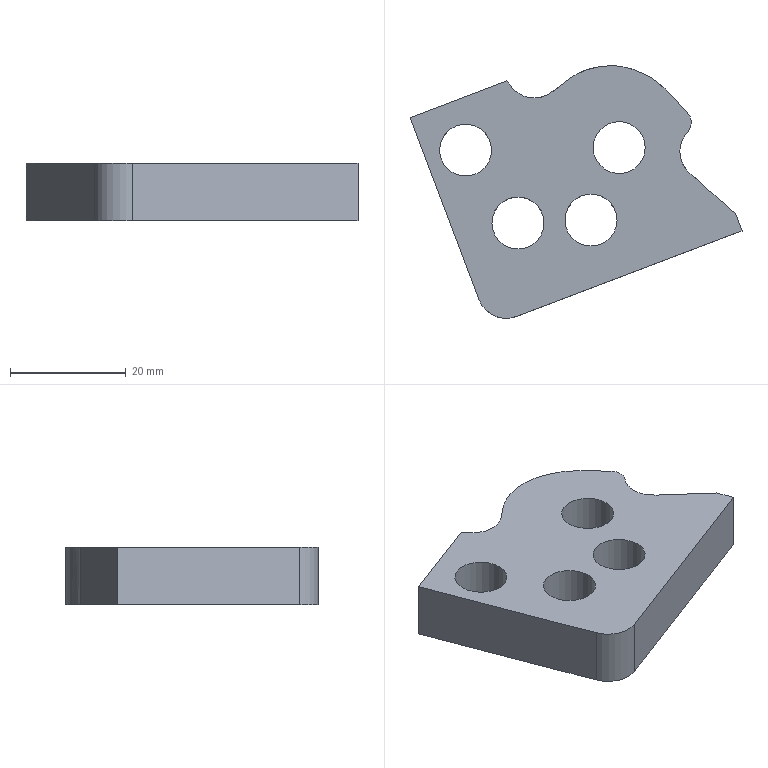Part | NX | features solid 2 | 1 solid | 16 faces | box 57.426 x 43.7 x 10 mm | volume 13256 mm3 | plane 7 | cylinder 5 | spline 4 | commonest cylinder face diameters 9 x4 10 x1
STEP:
#1=CARTESIAN_POINT('',(3760.865,-33.92,-118.));
#2=VERTEX_POINT('',#1);
#3=CARTESIAN_POINT('',(3760.865,-33.92,-128.));
#4=VERTEX_POINT('',#3);
#5=CARTESIAN_POINT('',(3760.865,-33.92,-123.));
#6=DIRECTION('',(0.,0.,-1.));
#7=VECTOR('',#6,1000.);
#8=LINE('',#5,#7);
#9=EDGE_CURVE('',#2,#4,#8,.T.);
#10=ORIENTED_EDGE('',*,*,#9,.T.);
#11=CARTESIAN_POINT('',(3754.535,-29.671,-128.));
#12=VERTEX_POINT('',#11);
#13=CARTESIAN_POINT('',(3760.865,-33.92,-128.));
#14=CARTESIAN_POINT('',(3760.334,-33.554,-128.));
#15=CARTESIAN_POINT('',(3759.497,-32.569,-128.));
#16=CARTESIAN_POINT('',(3758.35,-31.697,-128.));
#17=CARTESIAN_POINT('',(3757.593,-31.103,-128.));
#18=CARTESIAN_POINT('',(3756.992,-30.861,-128.));
#19=CARTESIAN_POINT('',(3756.278,-30.496,-128.));
#20=CARTESIAN_POINT('',(3755.398,-30.101,-128.));
#21=CARTESIAN_POINT('',(3754.834,-29.79,-128.));
#22=CARTESIAN_POINT('',(3754.535,-29.671,-128.));
#23=B_SPLINE_CURVE_WITH_KNOTS('',3,(#13,#14,#15,#16,#17,#18,#19,#20,#21,#22),.UNSPECIFIED.,.F.,.F.,(4,1,1,1,1,1,1,4),(0.,0.00192,0.003839,0.004319,0.004799,0.005759,0.006719,0.007679),.UNSPECIFIED.);
#24=EDGE_CURVE('',#4,#12,#23,.T.);
#25=ORIENTED_EDGE('',*,*,#24,.T.);
#26=CARTESIAN_POINT('',(3754.535,-29.671,-118.));
#27=VERTEX_POINT('',#26);
#28=CARTESIAN_POINT('',(3754.535,-29.671,-128.));
#29=DIRECTION('',(0.,0.,1.));
#30=VECTOR('',#29,1000.);
#31=LINE('',#28,#30);
#32=EDGE_CURVE('',#12,#27,#31,.T.);
#33=ORIENTED_EDGE('',*,*,#32,.T.);
#34=CARTESIAN_POINT('',(3754.535,-29.671,-118.));
#35=CARTESIAN_POINT('',(3754.834,-29.79,-118.));
#36=CARTESIAN_POINT('',(3755.398,-30.1,-118.));
#37=CARTESIAN_POINT('',(3756.278,-30.496,-118.));
#38=CARTESIAN_POINT('',(3756.99,-30.86,-118.));
#39=CARTESIAN_POINT('',(3757.593,-31.103,-118.));
#40=CARTESIAN_POINT('',(3758.343,-31.692,-118.));
#41=CARTESIAN_POINT('',(3759.486,-32.558,-118.));
#42=CARTESIAN_POINT('',(3760.331,-33.552,-118.));
#43=CARTESIAN_POINT('',(3760.865,-33.92,-118.));
#44=B_SPLINE_CURVE_WITH_KNOTS('',3,(#34,#35,#36,#37,#38,#39,#40,#41,#42,#43),.UNSPECIFIED.,.F.,.F.,(4,1,1,1,1,1,1,4),(0.,0.0009638,0.001928,0.002891,0.003373,0.003855,0.005783,0.007711),.UNSPECIFIED.);
#45=EDGE_CURVE('',#27,#2,#44,.T.);
#46=ORIENTED_EDGE('',*,*,#45,.T.);
#47=EDGE_LOOP('',(#10,#25,#33,#46));
#48=FACE_BOUND('',#47,.T.);
#49=CARTESIAN_POINT('',(3760.865,-33.92,-128.));
#50=CARTESIAN_POINT('',(3760.865,-33.92,-118.));
#51=CARTESIAN_POINT('',(3760.682,-33.794,-128.));
#52=CARTESIAN_POINT('',(3760.682,-33.794,-118.));
#53=CARTESIAN_POINT('',(3760.52,-33.668,-128.));
#54=CARTESIAN_POINT('',(3760.52,-33.668,-118.));
#55=CARTESIAN_POINT('',(3760.266,-33.422,-128.));
#56=CARTESIAN_POINT('',(3760.266,-33.422,-118.));
#57=CARTESIAN_POINT('',(3760.189,-33.337,-128.));
#58=CARTESIAN_POINT('',(3760.189,-33.337,-118.));
#59=CARTESIAN_POINT('',(3760.086,-33.225,-128.));
#60=CARTESIAN_POINT('',(3760.086,-33.225,-118.));
#61=CARTESIAN_POINT('',(3760.058,-33.196,-128.));
#62=CARTESIAN_POINT('',(3760.058,-33.196,-118.));
#63=CARTESIAN_POINT('',(3759.912,-33.056,-128.));
#64=CARTESIAN_POINT('',(3759.912,-33.056,-118.));
#65=CARTESIAN_POINT('',(3759.775,-32.928,-128.));
#66=CARTESIAN_POINT('',(3759.775,-32.928,-118.));
#67=CARTESIAN_POINT('',(3759.532,-32.698,-128.));
#68=CARTESIAN_POINT('',(3759.532,-32.698,-118.));
#69=CARTESIAN_POINT('',(3759.413,-32.585,-128.));
#70=CARTESIAN_POINT('',(3759.413,-32.585,-118.));
#71=CARTESIAN_POINT('',(3759.237,-32.42,-128.));
#72=CARTESIAN_POINT('',(3759.237,-32.42,-118.));
#73=CARTESIAN_POINT('',(3759.164,-32.35,-128.));
#74=CARTESIAN_POINT('',(3759.164,-32.35,-118.));
#75=CARTESIAN_POINT('',(3759.04,-32.23,-128.));
#76=CARTESIAN_POINT('',(3759.04,-32.23,-118.));
#77=CARTESIAN_POINT('',(3759.001,-32.193,-128.));
#78=CARTESIAN_POINT('',(3759.001,-32.193,-118.));
#79=CARTESIAN_POINT('',(3758.932,-32.133,-128.));
#80=CARTESIAN_POINT('',(3758.932,-32.133,-118.));
#81=CARTESIAN_POINT('',(3758.892,-32.103,-128.));
#82=CARTESIAN_POINT('',(3758.892,-32.103,-118.));
#83=CARTESIAN_POINT('',(3758.763,-32.007,-128.));
#84=CARTESIAN_POINT('',(3758.763,-32.007,-118.));
#85=CARTESIAN_POINT('',(3758.683,-31.946,-128.));
#86=CARTESIAN_POINT('',(3758.683,-31.946,-118.));
#87=CARTESIAN_POINT('',(3758.355,-31.692,-128.));
#88=CARTESIAN_POINT('',(3758.355,-31.692,-118.));
#89=CARTESIAN_POINT('',(3758.093,-31.494,-128.));
#90=CARTESIAN_POINT('',(3758.093,-31.494,-118.));
#91=CARTESIAN_POINT('',(3757.712,-31.199,-128.));
#92=CARTESIAN_POINT('',(3757.712,-31.199,-118.));
#93=CARTESIAN_POINT('',(3757.664,-31.164,-128.));
#94=CARTESIAN_POINT('',(3757.664,-31.164,-118.));
#95=CARTESIAN_POINT('',(3757.523,-31.093,-128.));
#96=CARTESIAN_POINT('',(3757.523,-31.093,-118.));
#97=CARTESIAN_POINT('',(3757.304,-30.994,-128.));
#98=CARTESIAN_POINT('',(3757.304,-30.994,-118.));
#99=CARTESIAN_POINT('',(3756.869,-30.784,-128.));
#100=CARTESIAN_POINT('',(3756.869,-30.784,-118.));
#101=CARTESIAN_POINT('',(3756.567,-30.642,-128.));
#102=CARTESIAN_POINT('',(3756.567,-30.642,-118.));
#103=CARTESIAN_POINT('',(3755.969,-30.358,-128.));
#104=CARTESIAN_POINT('',(3755.969,-30.358,-118.));
#105=CARTESIAN_POINT('',(3755.668,-30.215,-128.));
#106=CARTESIAN_POINT('',(3755.668,-30.215,-118.));
#107=CARTESIAN_POINT('',(3755.222,-30.002,-128.));
#108=CARTESIAN_POINT('',(3755.222,-30.002,-118.));
#109=CARTESIAN_POINT('',(3755.074,-29.932,-128.));
#110=CARTESIAN_POINT('',(3755.074,-29.932,-118.));
#111=CARTESIAN_POINT('',(3754.853,-29.829,-128.));
#112=CARTESIAN_POINT('',(3754.853,-29.829,-118.));
#113=CARTESIAN_POINT('',(3754.76,-29.786,-128.));
#114=CARTESIAN_POINT('',(3754.76,-29.786,-118.));
#115=CARTESIAN_POINT('',(3754.58,-29.694,-128.));
#116=CARTESIAN_POINT('',(3754.58,-29.694,-118.));
#117=CARTESIAN_POINT('',(3754.538,-29.672,-128.));
#118=CARTESIAN_POINT('',(3754.538,-29.672,-118.));
#119=CARTESIAN_POINT('',(3754.535,-29.671,-128.));
#120=CARTESIAN_POINT('',(3754.535,-29.671,-118.));
#121=B_SPLINE_SURFACE_WITH_KNOTS('',3,1,((#49,#50),(#51,#52),(#53,#54),(#55,#56),(#57,#58),(#59,#60),(#61,#62),(#63,#64),(#65,#66),(#67,#68),(#69,#70),(#71,#72),(#73,#74),(#75,#76),(#77,#78),(#79,#80),(#81,#82),(#83,#84),(#85,#86),(#87,#88),(#89,#90),(#91,#92),(#93,#94),(#95,#96),(#97,#98),(#99,#100),(#101,#102),(#103,#104),(#105,#106),(#107,#108),(#109,#110),(#111,#112),(#113,#114),(#115,#116),(#117,#118),(#119,#120)),.SURF_OF_LINEAR_EXTRUSION.,.F.,.F.,.F.,(4,2,2,2,2,2,2,2,2,2,2,2,2,2,2,2,2,4),(2,2),(0.,0.0625,0.09375,0.125,0.1875,0.25,0.2812,0.3125,0.3438,0.375,0.5,0.5625,0.625,0.75,0.875,0.9375,0.9688,1.),(0.,1.),.UNSPECIFIED.);
#122=ADVANCED_FACE('',(#48),#121,.T.);
#123=CARTESIAN_POINT('',(3763.834,-37.209,-128.));
#124=VERTEX_POINT('',#123);
#125=CARTESIAN_POINT('',(3763.86,-40.309,-128.));
#126=VERTEX_POINT('',#125);
#127=CARTESIAN_POINT('',(3763.834,-37.209,-128.));
#128=CARTESIAN_POINT('',(3764.598,-38.056,-128.));
#129=CARTESIAN_POINT('',(3764.61,-39.451,-128.));
#130=CARTESIAN_POINT('',(3763.86,-40.309,-128.));
#131=B_SPLINE_CURVE_WITH_KNOTS('',3,(#127,#128,#129,#130),.UNSPECIFIED.,.F.,.F.,(4,4),(0.,0.003372),.UNSPECIFIED.);
#132=EDGE_CURVE('',#124,#126,#131,.T.);
#133=ORIENTED_EDGE('',*,*,#132,.T.);
#134=CARTESIAN_POINT('',(3772.059,-54.603,-128.));
#135=VERTEX_POINT('',#134);
#136=CARTESIAN_POINT('',(3772.059,-54.603,-128.));
#137=CARTESIAN_POINT('',(3770.892,-53.566,-128.));
#138=CARTESIAN_POINT('',(3769.143,-52.009,-128.));
#139=CARTESIAN_POINT('',(3766.801,-49.941,-128.));
#140=CARTESIAN_POINT('',(3765.071,-48.37,-128.));
#141=CARTESIAN_POINT('',(3763.239,-46.871,-128.));
#142=CARTESIAN_POINT('',(3762.327,-44.647,-128.));
#143=CARTESIAN_POINT('',(3762.484,-42.239,-128.));
#144=CARTESIAN_POINT('',(3763.338,-40.894,-128.));
#145=CARTESIAN_POINT('',(3763.86,-40.309,-128.));
#146=B_SPLINE_CURVE_WITH_KNOTS('',3,(#136,#137,#138,#139,#140,#141,#142,#143,#144,#145),.UNSPECIFIED.,.F.,.F.,(4,1,1,1,1,1,1,4),(0.,0.004684,0.007026,0.009369,0.01171,0.01405,0.0164,0.01874),.UNSPECIFIED.);
#147=EDGE_CURVE('',#135,#126,#146,.T.);
#148=ORIENTED_EDGE('',*,*,#147,.F.);
#149=CARTESIAN_POINT('',(3773.182,-57.565,-128.));
#150=VERTEX_POINT('',#149);
#151=CARTESIAN_POINT('',(3765.144,-36.356,-128.));
#152=DIRECTION('',(-0.3544,0.9351,0.));
#153=VECTOR('',#152,1000.);
#154=LINE('',#151,#153);
#155=EDGE_CURVE('',#150,#135,#154,.T.);
#156=ORIENTED_EDGE('',*,*,#155,.F.);
#157=CARTESIAN_POINT('',(3734.136,-72.362,-128.));
#158=VERTEX_POINT('',#157);
#159=CARTESIAN_POINT('',(3764.628,-60.806,-128.));
#160=DIRECTION('',(0.9351,0.3544,0.));
#161=VECTOR('',#160,1000.);
#162=LINE('',#159,#161);
#163=EDGE_CURVE('',#158,#150,#162,.T.);
#164=ORIENTED_EDGE('',*,*,#163,.F.);
#165=CARTESIAN_POINT('',(3727.688,-69.459,-128.));
#166=VERTEX_POINT('',#165);
#167=CARTESIAN_POINT('',(3732.364,-67.687,-128.));
#168=DIRECTION('',(0.,0.,-1.));
#169=DIRECTION('',(-1.,0.,0.));
#170=AXIS2_PLACEMENT_3D('',#167,#168,#169);
#171=CIRCLE('',#170,5.);
#172=EDGE_CURVE('',#158,#166,#171,.T.);
#173=ORIENTED_EDGE('',*,*,#172,.T.);
#174=CARTESIAN_POINT('',(3715.755,-37.972,-128.));
#175=VERTEX_POINT('',#174);
#176=CARTESIAN_POINT('',(3721.722,-53.715,-128.));
#177=DIRECTION('',(0.3544,-0.9351,0.));
#178=VECTOR('',#177,1000.);
#179=LINE('',#176,#178);
#180=EDGE_CURVE('',#175,#166,#179,.T.);
#181=ORIENTED_EDGE('',*,*,#180,.F.);
#182=CARTESIAN_POINT('',(3732.503,-31.625,-128.));
#183=VERTEX_POINT('',#182);
#184=CARTESIAN_POINT('',(3731.676,-31.938,-128.));
#185=DIRECTION('',(-0.9351,-0.3544,0.));
#186=VECTOR('',#185,1000.);
#187=LINE('',#184,#186);
#188=EDGE_CURVE('',#183,#175,#187,.T.);
#189=ORIENTED_EDGE('',*,*,#188,.F.);
#190=CARTESIAN_POINT('',(3754.535,-29.671,-128.));
#191=CARTESIAN_POINT('',(3754.294,-29.585,-128.));
#192=CARTESIAN_POINT('',(3753.792,-29.49,-128.));
#193=CARTESIAN_POINT('',(3752.817,-29.169,-128.));
#194=CARTESIAN_POINT('',(3751.927,-29.13,-128.));
#195=CARTESIAN_POINT('',(3751.174,-28.978,-128.));
#196=CARTESIAN_POINT('',(3750.674,-29.016,-128.));
#197=CARTESIAN_POINT('',(3750.049,-29.03,-128.));
#198=CARTESIAN_POINT('',(3749.3,-29.075,-128.));
#199=CARTESIAN_POINT('',(3748.547,-29.062,-128.));
#200=CARTESIAN_POINT('',(3747.812,-29.312,-128.));
#201=CARTESIAN_POINT('',(3747.074,-29.496,-128.));
#202=CARTESIAN_POINT('',(3746.323,-29.655,-128.));
#203=CARTESIAN_POINT('',(3745.624,-29.976,-128.));
#204=CARTESIAN_POINT('',(3744.911,-30.273,-128.));
#205=CARTESIAN_POINT('',(3744.027,-30.777,-128.));
#206=CARTESIAN_POINT('',(3742.521,-31.724,-128.));
#207=CARTESIAN_POINT('',(3740.975,-33.089,-128.));
#208=CARTESIAN_POINT('',(3739.304,-34.251,-128.));
#209=CARTESIAN_POINT('',(3737.217,-34.786,-128.));
#210=CARTESIAN_POINT('',(3735.054,-34.31,-128.));
#211=CARTESIAN_POINT('',(3733.429,-32.917,-128.));
#212=CARTESIAN_POINT('',(3732.825,-32.044,-128.));
#213=CARTESIAN_POINT('',(3732.503,-31.625,-128.));
#214=B_SPLINE_CURVE_WITH_KNOTS('',3,(#190,#191,#192,#193,#194,#195,#196,#197,#198,#199,#200,#201,#202,#203,#204,#205,#206,#207,#208,#209,#210,#211,#212,#213),.UNSPECIFIED.,.F.,.F.,(4,1,1,1,1,1,1,1,1,1,1,1,1,1,1,1,1,1,1,1,1,4),(0.,0.0007655,0.001531,0.003062,0.003445,0.003828,0.004593,0.005359,0.006124,0.00689,0.007655,0.008421,0.009186,0.009952,0.01072,0.01225,0.01531,0.01684,0.01837,0.02143,0.02297,0.0245),.UNSPECIFIED.);
#215=EDGE_CURVE('',#12,#183,#214,.T.);
#216=ORIENTED_EDGE('',*,*,#215,.F.);
#217=ORIENTED_EDGE('',*,*,#24,.F.);
#218=CARTESIAN_POINT('',(3763.834,-37.209,-128.));
#219=DIRECTION('',(-0.6701,0.7423,0.));
#220=VECTOR('',#219,1000.);
#221=LINE('',#218,#220);
#222=EDGE_CURVE('',#124,#4,#221,.T.);
#223=ORIENTED_EDGE('',*,*,#222,.F.);
#224=EDGE_LOOP('',(#133,#148,#156,#164,#173,#181,#189,#216,#217,#223));
#225=FACE_BOUND('',#224,.T.);
#226=CARTESIAN_POINT('',(3729.93,-56.209,-128.));
#227=VERTEX_POINT('',#226);
#228=CARTESIAN_POINT('',(3734.43,-56.209,-128.));
#229=DIRECTION('',(0.,0.,-1.));
#230=DIRECTION('',(-1.,0.,0.));
#231=AXIS2_PLACEMENT_3D('',#228,#229,#230);
#232=CIRCLE('',#231,4.5);
#233=EDGE_CURVE('',#227,#227,#232,.T.);
#234=ORIENTED_EDGE('',*,*,#233,.F.);
#235=EDGE_LOOP('',(#234));
#236=FACE_BOUND('',#235,.T.);
#237=CARTESIAN_POINT('',(3742.569,-55.697,-128.));
#238=VERTEX_POINT('',#237);
#239=CARTESIAN_POINT('',(3747.069,-55.697,-128.));
#240=DIRECTION('',(0.,0.,-1.));
#241=DIRECTION('',(-1.,0.,0.));
#242=AXIS2_PLACEMENT_3D('',#239,#240,#241);
#243=CIRCLE('',#242,4.5);
#244=EDGE_CURVE('',#238,#238,#243,.T.);
#245=ORIENTED_EDGE('',*,*,#244,.F.);
#246=EDGE_LOOP('',(#245));
#247=FACE_BOUND('',#246,.T.);
#248=CARTESIAN_POINT('',(3720.874,-43.601,-128.));
#249=VERTEX_POINT('',#248);
#250=CARTESIAN_POINT('',(3725.374,-43.601,-128.));
#251=DIRECTION('',(0.,0.,-1.));
#252=DIRECTION('',(-1.,0.,0.));
#253=AXIS2_PLACEMENT_3D('',#250,#251,#252);
#254=CIRCLE('',#253,4.5);
#255=EDGE_CURVE('',#249,#249,#254,.T.);
#256=ORIENTED_EDGE('',*,*,#255,.F.);
#257=EDGE_LOOP('',(#256));
#258=FACE_BOUND('',#257,.T.);
#259=CARTESIAN_POINT('',(3747.441,-43.157,-128.));
#260=VERTEX_POINT('',#259);
#261=CARTESIAN_POINT('',(3751.941,-43.157,-128.));
#262=DIRECTION('',(0.,0.,-1.));
#263=DIRECTION('',(-1.,0.,0.));
#264=AXIS2_PLACEMENT_3D('',#261,#262,#263);
#265=CIRCLE('',#264,4.5);
#266=EDGE_CURVE('',#260,#260,#265,.T.);
#267=ORIENTED_EDGE('',*,*,#266,.F.);
#268=EDGE_LOOP('',(#267));
#269=FACE_BOUND('',#268,.T.);
#270=CARTESIAN_POINT('',(1974.5,193.,-128.));
#271=DIRECTION('',(0.,0.,-1.));
#272=DIRECTION('',(-1.,0.,0.));
#273=AXIS2_PLACEMENT_3D('',#270,#271,#272);
#274=PLANE('',#273);
#275=ADVANCED_FACE('',(#225,#236,#247,#258,#269),#274,.T.);
#276=CARTESIAN_POINT('',(3729.93,-56.209,-118.));
#277=VERTEX_POINT('',#276);
#278=CARTESIAN_POINT('',(3734.43,-56.209,-118.));
#279=DIRECTION('',(0.,0.,-1.));
#280=DIRECTION('',(-1.,0.,0.));
#281=AXIS2_PLACEMENT_3D('',#278,#279,#280);
#282=CIRCLE('',#281,4.5);
#283=EDGE_CURVE('',#277,#277,#282,.T.);
#284=ORIENTED_EDGE('',*,*,#283,.T.);
#285=EDGE_LOOP('',(#284));
#286=FACE_BOUND('',#285,.T.);
#287=CARTESIAN_POINT('',(3742.569,-55.697,-118.));
#288=VERTEX_POINT('',#287);
#289=CARTESIAN_POINT('',(3747.069,-55.697,-118.));
#290=DIRECTION('',(0.,0.,-1.));
#291=DIRECTION('',(-1.,0.,0.));
#292=AXIS2_PLACEMENT_3D('',#289,#290,#291);
#293=CIRCLE('',#292,4.5);
#294=EDGE_CURVE('',#288,#288,#293,.T.);
#295=ORIENTED_EDGE('',*,*,#294,.T.);
#296=EDGE_LOOP('',(#295));
#297=FACE_BOUND('',#296,.T.);
#298=CARTESIAN_POINT('',(3720.874,-43.601,-118.));
#299=VERTEX_POINT('',#298);
#300=CARTESIAN_POINT('',(3725.374,-43.601,-118.));
#301=DIRECTION('',(0.,0.,-1.));
#302=DIRECTION('',(-1.,0.,0.));
#303=AXIS2_PLACEMENT_3D('',#300,#301,#302);
#304=CIRCLE('',#303,4.5);
#305=EDGE_CURVE('',#299,#299,#304,.T.);
#306=ORIENTED_EDGE('',*,*,#305,.T.);
#307=EDGE_LOOP('',(#306));
#308=FACE_BOUND('',#307,.T.);
#309=CARTESIAN_POINT('',(3747.441,-43.157,-118.));
#310=VERTEX_POINT('',#309);
#311=CARTESIAN_POINT('',(3751.941,-43.157,-118.));
#312=DIRECTION('',(0.,0.,-1.));
#313=DIRECTION('',(-1.,0.,0.));
#314=AXIS2_PLACEMENT_3D('',#311,#312,#313);
#315=CIRCLE('',#314,4.5);
#316=EDGE_CURVE('',#310,#310,#315,.T.);
#317=ORIENTED_EDGE('',*,*,#316,.T.);
#318=EDGE_LOOP('',(#317));
#319=FACE_BOUND('',#318,.T.);
#320=CARTESIAN_POINT('',(3763.834,-37.209,-118.));
#321=VERTEX_POINT('',#320);
#322=CARTESIAN_POINT('',(3763.834,-37.209,-118.));
#323=DIRECTION('',(-0.6701,0.7423,0.));
#324=VECTOR('',#323,1000.);
#325=LINE('',#322,#324);
#326=EDGE_CURVE('',#321,#2,#325,.T.);
#327=ORIENTED_EDGE('',*,*,#326,.T.);
#328=ORIENTED_EDGE('',*,*,#45,.F.);
#329=CARTESIAN_POINT('',(3732.503,-31.625,-118.));
#330=VERTEX_POINT('',#329);
#331=CARTESIAN_POINT('',(3732.503,-31.625,-118.));
#332=CARTESIAN_POINT('',(3732.813,-32.029,-118.));
#333=CARTESIAN_POINT('',(3733.396,-32.866,-118.));
#334=CARTESIAN_POINT('',(3734.935,-34.24,-118.));
#335=CARTESIAN_POINT('',(3737.,-34.765,-118.));
#336=CARTESIAN_POINT('',(3739.029,-34.357,-118.));
#337=CARTESIAN_POINT('',(3740.341,-33.571,-118.));
#338=CARTESIAN_POINT('',(3741.532,-32.58,-118.));
#339=CARTESIAN_POINT('',(3742.553,-31.802,-118.));
#340=CARTESIAN_POINT('',(3743.361,-31.166,-118.));
#341=CARTESIAN_POINT('',(3744.039,-30.796,-118.));
#342=CARTESIAN_POINT('',(3744.676,-30.363,-118.));
#343=CARTESIAN_POINT('',(3745.411,-30.085,-118.));
#344=CARTESIAN_POINT('',(3746.104,-29.714,-118.));
#345=CARTESIAN_POINT('',(3746.865,-29.55,-118.));
#346=CARTESIAN_POINT('',(3747.615,-29.357,-118.));
#347=CARTESIAN_POINT('',(3748.607,-29.06,-118.));
#348=CARTESIAN_POINT('',(3749.667,-29.046,-118.));
#349=CARTESIAN_POINT('',(3750.58,-29.027,-118.));
#350=CARTESIAN_POINT('',(3751.109,-28.967,-118.));
#351=CARTESIAN_POINT('',(3751.617,-29.072,-118.));
#352=CARTESIAN_POINT('',(3752.258,-29.15,-118.));
#353=CARTESIAN_POINT('',(3753.029,-29.237,-118.));
#354=CARTESIAN_POINT('',(3753.776,-29.486,-118.));
#355=CARTESIAN_POINT('',(3754.289,-29.583,-118.));
#356=CARTESIAN_POINT('',(3754.535,-29.671,-118.));
#357=B_SPLINE_CURVE_WITH_KNOTS('',3,(#331,#332,#333,#334,#335,#336,#337,#338,#339,#340,#341,#342,#343,#344,#345,#346,#347,#348,#349,#350,#351,#352,#353,#354,#355,#356),.UNSPECIFIED.,.F.,.F.,(4,1,1,1,1,1,1,1,1,1,1,1,1,1,1,1,1,1,1,1,1,1,1,4),(0.,0.001526,0.003052,0.006104,0.00763,0.009156,0.01068,0.01221,0.01297,0.01373,0.0145,0.01526,0.01602,0.01679,0.01755,0.01831,0.01984,0.0206,0.02098,0.02136,0.02213,0.02289,0.02365,0.02441),.UNSPECIFIED.);
#358=EDGE_CURVE('',#330,#27,#357,.T.);
#359=ORIENTED_EDGE('',*,*,#358,.F.);
#360=CARTESIAN_POINT('',(3715.755,-37.972,-118.));
#361=VERTEX_POINT('',#360);
#362=CARTESIAN_POINT('',(3731.676,-31.938,-118.));
#363=DIRECTION('',(-0.9351,-0.3544,0.));
#364=VECTOR('',#363,1000.);
#365=LINE('',#362,#364);
#366=EDGE_CURVE('',#330,#361,#365,.T.);
#367=ORIENTED_EDGE('',*,*,#366,.T.);
#368=CARTESIAN_POINT('',(3727.688,-69.459,-118.));
#369=VERTEX_POINT('',#368);
#370=CARTESIAN_POINT('',(3721.722,-53.715,-118.));
#371=DIRECTION('',(0.3544,-0.9351,0.));
#372=VECTOR('',#371,1000.);
#373=LINE('',#370,#372);
#374=EDGE_CURVE('',#361,#369,#373,.T.);
#375=ORIENTED_EDGE('',*,*,#374,.T.);
#376=CARTESIAN_POINT('',(3734.136,-72.362,-118.));
#377=VERTEX_POINT('',#376);
#378=CARTESIAN_POINT('',(3732.364,-67.687,-118.));
#379=DIRECTION('',(0.,0.,-1.));
#380=DIRECTION('',(-1.,0.,0.));
#381=AXIS2_PLACEMENT_3D('',#378,#379,#380);
#382=CIRCLE('',#381,5.);
#383=EDGE_CURVE('',#377,#369,#382,.T.);
#384=ORIENTED_EDGE('',*,*,#383,.F.);
#385=CARTESIAN_POINT('',(3773.182,-57.565,-118.));
#386=VERTEX_POINT('',#385);
#387=CARTESIAN_POINT('',(3764.628,-60.806,-118.));
#388=DIRECTION('',(0.9351,0.3544,0.));
#389=VECTOR('',#388,1000.);
#390=LINE('',#387,#389);
#391=EDGE_CURVE('',#377,#386,#390,.T.);
#392=ORIENTED_EDGE('',*,*,#391,.T.);
#393=CARTESIAN_POINT('',(3772.059,-54.603,-118.));
#394=VERTEX_POINT('',#393);
#395=CARTESIAN_POINT('',(3765.144,-36.356,-118.));
#396=DIRECTION('',(-0.3544,0.9351,0.));
#397=VECTOR('',#396,1000.);
#398=LINE('',#395,#397);
#399=EDGE_CURVE('',#386,#394,#398,.T.);
#400=ORIENTED_EDGE('',*,*,#399,.T.);
#401=CARTESIAN_POINT('',(3763.86,-40.309,-118.));
#402=VERTEX_POINT('',#401);
#403=CARTESIAN_POINT('',(3763.86,-40.309,-118.));
#404=CARTESIAN_POINT('',(3763.337,-40.895,-118.));
#405=CARTESIAN_POINT('',(3762.483,-42.244,-118.));
#406=CARTESIAN_POINT('',(3762.325,-44.652,-118.));
#407=CARTESIAN_POINT('',(3763.256,-46.896,-118.));
#408=CARTESIAN_POINT('',(3765.099,-48.392,-118.));
#409=CARTESIAN_POINT('',(3766.818,-49.956,-118.));
#410=CARTESIAN_POINT('',(3769.153,-52.018,-118.));
#411=CARTESIAN_POINT('',(3770.895,-53.57,-118.));
#412=CARTESIAN_POINT('',(3772.059,-54.603,-118.));
#413=B_SPLINE_CURVE_WITH_KNOTS('',3,(#403,#404,#405,#406,#407,#408,#409,#410,#411,#412),.UNSPECIFIED.,.F.,.F.,(4,1,1,1,1,1,1,4),(0.,0.002332,0.004664,0.006996,0.009328,0.01166,0.01399,0.01866),.UNSPECIFIED.);
#414=EDGE_CURVE('',#402,#394,#413,.T.);
#415=ORIENTED_EDGE('',*,*,#414,.F.);
#416=CARTESIAN_POINT('',(3763.834,-37.209,-118.));
#417=CARTESIAN_POINT('',(3764.598,-38.056,-118.));
#418=CARTESIAN_POINT('',(3764.61,-39.451,-118.));
#419=CARTESIAN_POINT('',(3763.86,-40.309,-118.));
#420=B_SPLINE_CURVE_WITH_KNOTS('',3,(#416,#417,#418,#419),.UNSPECIFIED.,.F.,.F.,(4,4),(0.,0.003372),.UNSPECIFIED.);
#421=EDGE_CURVE('',#321,#402,#420,.T.);
#422=ORIENTED_EDGE('',*,*,#421,.F.);
#423=EDGE_LOOP('',(#327,#328,#359,#367,#375,#384,#392,#400,#415,#422));
#424=FACE_BOUND('',#423,.T.);
#425=CARTESIAN_POINT('',(1974.5,193.,-118.));
#426=DIRECTION('',(0.,0.,-1.));
#427=DIRECTION('',(-1.,0.,0.));
#428=AXIS2_PLACEMENT_3D('',#425,#426,#427);
#429=PLANE('',#428);
#430=ADVANCED_FACE('',(#286,#297,#308,#319,#424),#429,.F.);
#431=CARTESIAN_POINT('',(3763.86,-40.309,-123.));
#432=DIRECTION('',(0.,0.,1.));
#433=VECTOR('',#432,1000.);
#434=LINE('',#431,#433);
#435=EDGE_CURVE('',#126,#402,#434,.T.);
#436=ORIENTED_EDGE('',*,*,#435,.T.);
#437=ORIENTED_EDGE('',*,*,#414,.T.);
#438=CARTESIAN_POINT('',(3772.059,-54.603,-123.));
#439=DIRECTION('',(0.,0.,-1.));
#440=VECTOR('',#439,1000.);
#441=LINE('',#438,#440);
#442=EDGE_CURVE('',#394,#135,#441,.T.);
#443=ORIENTED_EDGE('',*,*,#442,.T.);
#444=ORIENTED_EDGE('',*,*,#147,.T.);
#445=EDGE_LOOP('',(#436,#437,#443,#444));
#446=FACE_BOUND('',#445,.T.);
#447=CARTESIAN_POINT('',(3772.059,-54.603,-128.));
#448=CARTESIAN_POINT('',(3772.059,-54.603,-118.));
#449=CARTESIAN_POINT('',(3769.934,-52.716,-128.));
#450=CARTESIAN_POINT('',(3769.934,-52.716,-118.));
#451=CARTESIAN_POINT('',(3767.809,-50.828,-128.));
#452=CARTESIAN_POINT('',(3767.809,-50.828,-118.));
#453=CARTESIAN_POINT('',(3765.419,-48.706,-128.));
#454=CARTESIAN_POINT('',(3765.419,-48.706,-118.));
#455=CARTESIAN_POINT('',(3765.154,-48.471,-128.));
#456=CARTESIAN_POINT('',(3765.154,-48.471,-118.));
#457=CARTESIAN_POINT('',(3764.755,-48.116,-128.));
#458=CARTESIAN_POINT('',(3764.755,-48.116,-118.));
#459=CARTESIAN_POINT('',(3764.623,-47.999,-128.));
#460=CARTESIAN_POINT('',(3764.623,-47.999,-118.));
#461=CARTESIAN_POINT('',(3764.355,-47.761,-128.));
#462=CARTESIAN_POINT('',(3764.355,-47.761,-118.));
#463=CARTESIAN_POINT('',(3764.233,-47.656,-128.));
#464=CARTESIAN_POINT('',(3764.233,-47.656,-118.));
#465=CARTESIAN_POINT('',(3763.928,-47.377,-128.));
#466=CARTESIAN_POINT('',(3763.928,-47.377,-118.));
#467=CARTESIAN_POINT('',(3763.768,-47.215,-128.));
#468=CARTESIAN_POINT('',(3763.768,-47.215,-118.));
#469=CARTESIAN_POINT('',(3763.475,-46.868,-128.));
#470=CARTESIAN_POINT('',(3763.475,-46.868,-118.));
#471=CARTESIAN_POINT('',(3763.347,-46.695,-128.));
#472=CARTESIAN_POINT('',(3763.347,-46.695,-118.));
#473=CARTESIAN_POINT('',(3762.969,-46.103,-128.));
#474=CARTESIAN_POINT('',(3762.969,-46.103,-118.));
#475=CARTESIAN_POINT('',(3762.785,-45.694,-128.));
#476=CARTESIAN_POINT('',(3762.785,-45.694,-118.));
#477=CARTESIAN_POINT('',(3762.397,-44.419,-128.));
#478=CARTESIAN_POINT('',(3762.397,-44.419,-118.));
#479=CARTESIAN_POINT('',(3762.368,-43.464,-128.));
#480=CARTESIAN_POINT('',(3762.368,-43.464,-118.));
#481=CARTESIAN_POINT('',(3762.702,-42.147,-128.));
#482=CARTESIAN_POINT('',(3762.702,-42.147,-118.));
#483=CARTESIAN_POINT('',(3762.873,-41.724,-128.));
#484=CARTESIAN_POINT('',(3762.873,-41.724,-118.));
#485=CARTESIAN_POINT('',(3763.318,-40.942,-128.));
#486=CARTESIAN_POINT('',(3763.318,-40.942,-118.));
#487=CARTESIAN_POINT('',(3763.617,-40.581,-128.));
#488=CARTESIAN_POINT('',(3763.617,-40.581,-118.));
#489=CARTESIAN_POINT('',(3763.86,-40.309,-128.));
#490=CARTESIAN_POINT('',(3763.86,-40.309,-118.));
#491=B_SPLINE_SURFACE_WITH_KNOTS('',3,1,((#447,#448),(#449,#450),(#451,#452),(#453,#454),(#455,#456),(#457,#458),(#459,#460),(#461,#462),(#463,#464),(#465,#466),(#467,#468),(#469,#470),(#471,#472),(#473,#474),(#475,#476),(#477,#478),(#479,#480),(#481,#482),(#483,#484),(#485,#486),(#487,#488),(#489,#490)),.SURF_OF_LINEAR_EXTRUSION.,.F.,.F.,.F.,(4,2,2,2,2,2,2,2,2,2,4),(2,2),(0.,0.5,0.5625,0.5937,0.625,0.6562,0.6875,0.75,0.875,0.9375,1.),(0.,1.),.UNSPECIFIED.);
#492=ADVANCED_FACE('',(#446),#491,.T.);
#493=CARTESIAN_POINT('',(3732.503,-31.625,-118.));
#494=DIRECTION('',(0.,0.,-1.));
#495=VECTOR('',#494,1000.);
#496=LINE('',#493,#495);
#497=EDGE_CURVE('',#330,#183,#496,.T.);
#498=ORIENTED_EDGE('',*,*,#497,.T.);
#499=ORIENTED_EDGE('',*,*,#188,.T.);
#500=CARTESIAN_POINT('',(3715.755,-37.972,-128.));
#501=DIRECTION('',(0.,0.,1.));
#502=VECTOR('',#501,1000.);
#503=LINE('',#500,#502);
#504=EDGE_CURVE('',#175,#361,#503,.T.);
#505=ORIENTED_EDGE('',*,*,#504,.T.);
#506=ORIENTED_EDGE('',*,*,#366,.F.);
#507=EDGE_LOOP('',(#498,#499,#505,#506));
#508=FACE_BOUND('',#507,.T.);
#509=CARTESIAN_POINT('',(3731.676,-31.938,-128.));
#510=DIRECTION('',(0.3544,-0.9351,0.));
#511=DIRECTION('',(0.9351,0.3544,0.));
#512=AXIS2_PLACEMENT_3D('',#509,#510,#511);
#513=PLANE('',#512);
#514=ADVANCED_FACE('',(#508),#513,.F.);
#515=ORIENTED_EDGE('',*,*,#442,.F.);
#516=ORIENTED_EDGE('',*,*,#399,.F.);
#517=CARTESIAN_POINT('',(3773.182,-57.565,-128.));
#518=DIRECTION('',(0.,0.,1.));
#519=VECTOR('',#518,1000.);
#520=LINE('',#517,#519);
#521=EDGE_CURVE('',#150,#386,#520,.T.);
#522=ORIENTED_EDGE('',*,*,#521,.F.);
#523=ORIENTED_EDGE('',*,*,#155,.T.);
#524=EDGE_LOOP('',(#515,#516,#522,#523));
#525=FACE_BOUND('',#524,.T.);
#526=CARTESIAN_POINT('',(3765.144,-36.356,-128.));
#527=DIRECTION('',(-0.9351,-0.3544,0.));
#528=DIRECTION('',(0.3544,-0.9351,0.));
#529=AXIS2_PLACEMENT_3D('',#526,#527,#528);
#530=PLANE('',#529);
#531=ADVANCED_FACE('',(#525),#530,.F.);
#532=ORIENTED_EDGE('',*,*,#374,.F.);
#533=ORIENTED_EDGE('',*,*,#504,.F.);
#534=ORIENTED_EDGE('',*,*,#180,.T.);
#535=CARTESIAN_POINT('',(3727.688,-69.459,-128.));
#536=DIRECTION('',(0.,0.,1.));
#537=VECTOR('',#536,1000.);
#538=LINE('',#535,#537);
#539=EDGE_CURVE('',#166,#369,#538,.T.);
#540=ORIENTED_EDGE('',*,*,#539,.T.);
#541=EDGE_LOOP('',(#532,#533,#534,#540));
#542=FACE_BOUND('',#541,.T.);
#543=CARTESIAN_POINT('',(3721.722,-53.715,-128.));
#544=DIRECTION('',(0.9351,0.3544,0.));
#545=DIRECTION('',(-0.3544,0.9351,0.));
#546=AXIS2_PLACEMENT_3D('',#543,#544,#545);
#547=PLANE('',#546);
#548=ADVANCED_FACE('',(#542),#547,.F.);
#549=ORIENTED_EDGE('',*,*,#383,.T.);
#550=ORIENTED_EDGE('',*,*,#539,.F.);
#551=ORIENTED_EDGE('',*,*,#172,.F.);
#552=CARTESIAN_POINT('',(3734.136,-72.362,-128.));
#553=DIRECTION('',(0.,0.,1.));
#554=VECTOR('',#553,1000.);
#555=LINE('',#552,#554);
#556=EDGE_CURVE('',#158,#377,#555,.T.);
#557=ORIENTED_EDGE('',*,*,#556,.T.);
#558=EDGE_LOOP('',(#549,#550,#551,#557));
#559=FACE_BOUND('',#558,.T.);
#560=CARTESIAN_POINT('',(3732.364,-67.687,-128.));
#561=DIRECTION('',(0.,0.,1.));
#562=DIRECTION('',(-1.,0.,0.));
#563=AXIS2_PLACEMENT_3D('',#560,#561,#562);
#564=CYLINDRICAL_SURFACE('',#563,5.);
#565=ADVANCED_FACE('',(#559),#564,.T.);
#566=ORIENTED_EDGE('',*,*,#391,.F.);
#567=ORIENTED_EDGE('',*,*,#556,.F.);
#568=ORIENTED_EDGE('',*,*,#163,.T.);
#569=ORIENTED_EDGE('',*,*,#521,.T.);
#570=EDGE_LOOP('',(#566,#567,#568,#569));
#571=FACE_BOUND('',#570,.T.);
#572=CARTESIAN_POINT('',(3764.628,-60.806,-128.));
#573=DIRECTION('',(-0.3544,0.9351,0.));
#574=DIRECTION('',(-0.9351,-0.3544,0.));
#575=AXIS2_PLACEMENT_3D('',#572,#573,#574);
#576=PLANE('',#575);
#577=ADVANCED_FACE('',(#571),#576,.F.);
#578=ORIENTED_EDGE('',*,*,#255,.T.);
#579=EDGE_LOOP('',(#578));
#580=FACE_BOUND('',#579,.T.);
#581=ORIENTED_EDGE('',*,*,#305,.F.);
#582=EDGE_LOOP('',(#581));
#583=FACE_BOUND('',#582,.T.);
#584=CARTESIAN_POINT('',(3725.374,-43.601,-128.));
#585=DIRECTION('',(0.,0.,1.));
#586=DIRECTION('',(-1.,0.,0.));
#587=AXIS2_PLACEMENT_3D('',#584,#585,#586);
#588=CYLINDRICAL_SURFACE('',#587,4.5);
#589=ADVANCED_FACE('',(#580,#583),#588,.F.);
#590=ORIENTED_EDGE('',*,*,#244,.T.);
#591=EDGE_LOOP('',(#590));
#592=FACE_BOUND('',#591,.T.);
#593=ORIENTED_EDGE('',*,*,#294,.F.);
#594=EDGE_LOOP('',(#593));
#595=FACE_BOUND('',#594,.T.);
#596=CARTESIAN_POINT('',(3747.069,-55.697,-128.));
#597=DIRECTION('',(0.,0.,1.));
#598=DIRECTION('',(-1.,0.,0.));
#599=AXIS2_PLACEMENT_3D('',#596,#597,#598);
#600=CYLINDRICAL_SURFACE('',#599,4.5);
#601=ADVANCED_FACE('',(#592,#595),#600,.F.);
#602=ORIENTED_EDGE('',*,*,#233,.T.);
#603=EDGE_LOOP('',(#602));
#604=FACE_BOUND('',#603,.T.);
#605=ORIENTED_EDGE('',*,*,#283,.F.);
#606=EDGE_LOOP('',(#605));
#607=FACE_BOUND('',#606,.T.);
#608=CARTESIAN_POINT('',(3734.43,-56.209,-128.));
#609=DIRECTION('',(0.,0.,1.));
#610=DIRECTION('',(-1.,0.,0.));
#611=AXIS2_PLACEMENT_3D('',#608,#609,#610);
#612=CYLINDRICAL_SURFACE('',#611,4.5);
#613=ADVANCED_FACE('',(#604,#607),#612,.F.);
#614=ORIENTED_EDGE('',*,*,#266,.T.);
#615=EDGE_LOOP('',(#614));
#616=FACE_BOUND('',#615,.T.);
#617=ORIENTED_EDGE('',*,*,#316,.F.);
#618=EDGE_LOOP('',(#617));
#619=FACE_BOUND('',#618,.T.);
#620=CARTESIAN_POINT('',(3751.941,-43.157,-128.));
#621=DIRECTION('',(0.,0.,1.));
#622=DIRECTION('',(-1.,0.,0.));
#623=AXIS2_PLACEMENT_3D('',#620,#621,#622);
#624=CYLINDRICAL_SURFACE('',#623,4.5);
#625=ADVANCED_FACE('',(#616,#619),#624,.F.);
#626=ORIENTED_EDGE('',*,*,#32,.F.);
#627=ORIENTED_EDGE('',*,*,#215,.T.);
#628=ORIENTED_EDGE('',*,*,#497,.F.);
#629=ORIENTED_EDGE('',*,*,#358,.T.);
#630=EDGE_LOOP('',(#626,#627,#628,#629));
#631=FACE_BOUND('',#630,.T.);
#632=CARTESIAN_POINT('',(3754.535,-29.671,-128.));
#633=CARTESIAN_POINT('',(3754.535,-29.671,-118.));
#634=CARTESIAN_POINT('',(3754.533,-29.671,-128.));
#635=CARTESIAN_POINT('',(3754.533,-29.671,-118.));
#636=CARTESIAN_POINT('',(3754.515,-29.665,-128.));
#637=CARTESIAN_POINT('',(3754.515,-29.665,-118.));
#638=CARTESIAN_POINT('',(3754.408,-29.639,-128.));
#639=CARTESIAN_POINT('',(3754.408,-29.639,-118.));
#640=CARTESIAN_POINT('',(3754.321,-29.619,-128.));
#641=CARTESIAN_POINT('',(3754.321,-29.619,-118.));
#642=CARTESIAN_POINT('',(3754.094,-29.557,-128.));
#643=CARTESIAN_POINT('',(3754.094,-29.557,-118.));
#644=CARTESIAN_POINT('',(3754.009,-29.531,-128.));
#645=CARTESIAN_POINT('',(3754.009,-29.531,-118.));
#646=CARTESIAN_POINT('',(3753.763,-29.465,-128.));
#647=CARTESIAN_POINT('',(3753.763,-29.465,-118.));
#648=CARTESIAN_POINT('',(3753.637,-29.429,-128.));
#649=CARTESIAN_POINT('',(3753.637,-29.429,-118.));
#650=CARTESIAN_POINT('',(3753.407,-29.367,-128.));
#651=CARTESIAN_POINT('',(3753.407,-29.367,-118.));
#652=CARTESIAN_POINT('',(3753.268,-29.329,-128.));
#653=CARTESIAN_POINT('',(3753.268,-29.329,-118.));
#654=CARTESIAN_POINT('',(3753.044,-29.268,-128.));
#655=CARTESIAN_POINT('',(3753.044,-29.268,-118.));
#656=CARTESIAN_POINT('',(3752.974,-29.25,-128.));
#657=CARTESIAN_POINT('',(3752.974,-29.25,-118.));
#658=CARTESIAN_POINT('',(3752.795,-29.22,-128.));
#659=CARTESIAN_POINT('',(3752.795,-29.22,-118.));
#660=CARTESIAN_POINT('',(3752.68,-29.206,-128.));
#661=CARTESIAN_POINT('',(3752.68,-29.206,-118.));
#662=CARTESIAN_POINT('',(3752.27,-29.152,-128.));
#663=CARTESIAN_POINT('',(3752.27,-29.152,-118.));
#664=CARTESIAN_POINT('',(3752.023,-29.116,-128.));
#665=CARTESIAN_POINT('',(3752.023,-29.116,-118.));
#666=CARTESIAN_POINT('',(3751.651,-29.063,-128.));
#667=CARTESIAN_POINT('',(3751.651,-29.063,-118.));
#668=CARTESIAN_POINT('',(3751.544,-29.05,-128.));
#669=CARTESIAN_POINT('',(3751.544,-29.05,-118.));
#670=CARTESIAN_POINT('',(3751.33,-29.02,-128.));
#671=CARTESIAN_POINT('',(3751.33,-29.02,-118.));
#672=CARTESIAN_POINT('',(3751.248,-29.007,-128.));
#673=CARTESIAN_POINT('',(3751.248,-29.007,-118.));
#674=CARTESIAN_POINT('',(3751.145,-28.991,-128.));
#675=CARTESIAN_POINT('',(3751.145,-28.991,-118.));
#676=CARTESIAN_POINT('',(3751.12,-28.988,-128.));
#677=CARTESIAN_POINT('',(3751.12,-28.988,-118.));
#678=CARTESIAN_POINT('',(3751.095,-28.987,-128.));
#679=CARTESIAN_POINT('',(3751.095,-28.987,-118.));
#680=CARTESIAN_POINT('',(3751.085,-28.987,-128.));
#681=CARTESIAN_POINT('',(3751.085,-28.987,-118.));
#682=CARTESIAN_POINT('',(3750.99,-28.993,-128.));
#683=CARTESIAN_POINT('',(3750.99,-28.993,-118.));
#684=CARTESIAN_POINT('',(3750.907,-28.999,-128.));
#685=CARTESIAN_POINT('',(3750.907,-28.999,-118.));
#686=CARTESIAN_POINT('',(3750.689,-29.01,-128.));
#687=CARTESIAN_POINT('',(3750.689,-29.01,-118.));
#688=CARTESIAN_POINT('',(3750.573,-29.011,-128.));
#689=CARTESIAN_POINT('',(3750.573,-29.011,-118.));
#690=CARTESIAN_POINT('',(3750.349,-29.022,-128.));
#691=CARTESIAN_POINT('',(3750.349,-29.022,-118.));
#692=CARTESIAN_POINT('',(3750.201,-29.028,-128.));
#693=CARTESIAN_POINT('',(3750.201,-29.028,-118.));
#694=CARTESIAN_POINT('',(3749.955,-29.038,-128.));
#695=CARTESIAN_POINT('',(3749.955,-29.038,-118.));
#696=CARTESIAN_POINT('',(3749.831,-29.044,-128.));
#697=CARTESIAN_POINT('',(3749.831,-29.044,-118.));
#698=CARTESIAN_POINT('',(3749.453,-29.059,-128.));
#699=CARTESIAN_POINT('',(3749.453,-29.059,-118.));
#700=CARTESIAN_POINT('',(3749.204,-29.068,-128.));
#701=CARTESIAN_POINT('',(3749.204,-29.068,-118.));
#702=CARTESIAN_POINT('',(3748.842,-29.085,-128.));
#703=CARTESIAN_POINT('',(3748.842,-29.085,-118.));
#704=CARTESIAN_POINT('',(3748.686,-29.09,-128.));
#705=CARTESIAN_POINT('',(3748.686,-29.09,-118.));
#706=CARTESIAN_POINT('',(3748.557,-29.1,-128.));
#707=CARTESIAN_POINT('',(3748.557,-29.1,-118.));
#708=CARTESIAN_POINT('',(3748.579,-29.098,-128.));
#709=CARTESIAN_POINT('',(3748.579,-29.098,-118.));
#710=CARTESIAN_POINT('',(3748.317,-29.172,-128.));
#711=CARTESIAN_POINT('',(3748.317,-29.172,-118.));
#712=CARTESIAN_POINT('',(3748.169,-29.209,-128.));
#713=CARTESIAN_POINT('',(3748.169,-29.209,-118.));
#714=CARTESIAN_POINT('',(3747.938,-29.267,-128.));
#715=CARTESIAN_POINT('',(3747.938,-29.267,-118.));
#716=CARTESIAN_POINT('',(3747.816,-29.3,-128.));
#717=CARTESIAN_POINT('',(3747.816,-29.3,-118.));
#718=CARTESIAN_POINT('',(3747.445,-29.396,-128.));
#719=CARTESIAN_POINT('',(3747.445,-29.396,-118.));
#720=CARTESIAN_POINT('',(3747.2,-29.459,-128.));
#721=CARTESIAN_POINT('',(3747.2,-29.459,-118.));
#722=CARTESIAN_POINT('',(3746.835,-29.553,-128.));
#723=CARTESIAN_POINT('',(3746.835,-29.553,-118.));
#724=CARTESIAN_POINT('',(3746.71,-29.585,-128.));
#725=CARTESIAN_POINT('',(3746.71,-29.585,-118.));
#726=CARTESIAN_POINT('',(3746.466,-29.647,-128.));
#727=CARTESIAN_POINT('',(3746.466,-29.647,-118.));
#728=CARTESIAN_POINT('',(3746.332,-29.681,-128.));
#729=CARTESIAN_POINT('',(3746.332,-29.681,-118.));
#730=CARTESIAN_POINT('',(3746.156,-29.731,-128.));
#731=CARTESIAN_POINT('',(3746.156,-29.731,-118.));
#732=CARTESIAN_POINT('',(3746.131,-29.74,-128.));
#733=CARTESIAN_POINT('',(3746.131,-29.74,-118.));
#734=CARTESIAN_POINT('',(3745.948,-29.824,-128.));
#735=CARTESIAN_POINT('',(3745.948,-29.824,-118.));
#736=CARTESIAN_POINT('',(3745.805,-29.89,-128.));
#737=CARTESIAN_POINT('',(3745.805,-29.89,-118.));
#738=CARTESIAN_POINT('',(3745.458,-30.044,-128.));
#739=CARTESIAN_POINT('',(3745.458,-30.044,-118.));
#740=CARTESIAN_POINT('',(3745.264,-30.133,-128.));
#741=CARTESIAN_POINT('',(3745.264,-30.133,-118.));
#742=CARTESIAN_POINT('',(3744.884,-30.303,-128.));
#743=CARTESIAN_POINT('',(3744.884,-30.303,-118.));
#744=CARTESIAN_POINT('',(3744.772,-30.348,-128.));
#745=CARTESIAN_POINT('',(3744.772,-30.348,-118.));
#746=CARTESIAN_POINT('',(3744.659,-30.405,-128.));
#747=CARTESIAN_POINT('',(3744.659,-30.405,-118.));
#748=CARTESIAN_POINT('',(3744.569,-30.461,-128.));
#749=CARTESIAN_POINT('',(3744.569,-30.461,-118.));
#750=CARTESIAN_POINT('',(3744.238,-30.662,-128.));
#751=CARTESIAN_POINT('',(3744.238,-30.662,-118.));
#752=CARTESIAN_POINT('',(3744.027,-30.788,-128.));
#753=CARTESIAN_POINT('',(3744.027,-30.788,-118.));
#754=CARTESIAN_POINT('',(3743.708,-30.981,-128.));
#755=CARTESIAN_POINT('',(3743.708,-30.981,-118.));
#756=CARTESIAN_POINT('',(3743.606,-31.043,-128.));
#757=CARTESIAN_POINT('',(3743.606,-31.043,-118.));
#758=CARTESIAN_POINT('',(3743.385,-31.177,-128.));
#759=CARTESIAN_POINT('',(3743.385,-31.177,-118.));
#760=CARTESIAN_POINT('',(3743.271,-31.244,-128.));
#761=CARTESIAN_POINT('',(3743.271,-31.244,-118.));
#762=CARTESIAN_POINT('',(3743.175,-31.309,-128.));
#763=CARTESIAN_POINT('',(3743.175,-31.309,-118.));
#764=CARTESIAN_POINT('',(3743.086,-31.382,-128.));
#765=CARTESIAN_POINT('',(3743.086,-31.382,-118.));
#766=CARTESIAN_POINT('',(3742.872,-31.551,-128.));
#767=CARTESIAN_POINT('',(3742.872,-31.551,-118.));
#768=CARTESIAN_POINT('',(3742.774,-31.626,-128.));
#769=CARTESIAN_POINT('',(3742.774,-31.626,-118.));
#770=CARTESIAN_POINT('',(3742.286,-32.006,-128.));
#771=CARTESIAN_POINT('',(3742.286,-32.006,-118.));
#772=CARTESIAN_POINT('',(3741.882,-32.321,-128.));
#773=CARTESIAN_POINT('',(3741.882,-32.321,-118.));
#774=CARTESIAN_POINT('',(3741.287,-32.784,-128.));
#775=CARTESIAN_POINT('',(3741.287,-32.784,-118.));
#776=CARTESIAN_POINT('',(3741.089,-32.939,-128.));
#777=CARTESIAN_POINT('',(3741.089,-32.939,-118.));
#778=CARTESIAN_POINT('',(3740.691,-33.249,-128.));
#779=CARTESIAN_POINT('',(3740.691,-33.249,-118.));
#780=CARTESIAN_POINT('',(3740.517,-33.388,-128.));
#781=CARTESIAN_POINT('',(3740.517,-33.388,-118.));
#782=CARTESIAN_POINT('',(3740.051,-33.741,-128.));
#783=CARTESIAN_POINT('',(3740.051,-33.741,-118.));
#784=CARTESIAN_POINT('',(3739.771,-33.92,-128.));
#785=CARTESIAN_POINT('',(3739.771,-33.92,-118.));
#786=CARTESIAN_POINT('',(3739.197,-34.207,-128.));
#787=CARTESIAN_POINT('',(3739.197,-34.207,-118.));
#788=CARTESIAN_POINT('',(3738.914,-34.317,-128.));
#789=CARTESIAN_POINT('',(3738.914,-34.317,-118.));
#790=CARTESIAN_POINT('',(3737.34,-34.755,-128.));
#791=CARTESIAN_POINT('',(3737.34,-34.755,-118.));
#792=CARTESIAN_POINT('',(3736.064,-34.608,-128.));
#793=CARTESIAN_POINT('',(3736.064,-34.608,-118.));
#794=CARTESIAN_POINT('',(3734.359,-33.72,-128.));
#795=CARTESIAN_POINT('',(3734.359,-33.72,-118.));
#796=CARTESIAN_POINT('',(3733.87,-33.325,-128.));
#797=CARTESIAN_POINT('',(3733.87,-33.325,-118.));
#798=CARTESIAN_POINT('',(3733.261,-32.618,-128.));
#799=CARTESIAN_POINT('',(3733.261,-32.618,-118.));
#800=CARTESIAN_POINT('',(3733.123,-32.426,-128.));
#801=CARTESIAN_POINT('',(3733.123,-32.426,-118.));
#802=CARTESIAN_POINT('',(3732.812,-32.026,-128.));
#803=CARTESIAN_POINT('',(3732.812,-32.026,-118.));
#804=CARTESIAN_POINT('',(3732.656,-31.824,-128.));
#805=CARTESIAN_POINT('',(3732.656,-31.824,-118.));
#806=CARTESIAN_POINT('',(3732.503,-31.625,-128.));
#807=CARTESIAN_POINT('',(3732.503,-31.625,-118.));
#808=B_SPLINE_SURFACE_WITH_KNOTS('',3,1,((#632,#633),(#634,#635),(#636,#637),(#638,#639),(#640,#641),(#642,#643),(#644,#645),(#646,#647),(#648,#649),(#650,#651),(#652,#653),(#654,#655),(#656,#657),(#658,#659),(#660,#661),(#662,#663),(#664,#665),(#666,#667),(#668,#669),(#670,#671),(#672,#673),(#674,#675),(#676,#677),(#678,#679),(#680,#681),(#682,#683),(#684,#685),(#686,#687),(#688,#689),(#690,#691),(#692,#693),(#694,#695),(#696,#697),(#698,#699),(#700,#701),(#702,#703),(#704,#705),(#706,#707),(#708,#709),(#710,#711),(#712,#713),(#714,#715),(#716,#717),(#718,#719),(#720,#721),(#722,#723),(#724,#725),(#726,#727),(#728,#729),(#730,#731),(#732,#733),(#734,#735),(#736,#737),(#738,#739),(#740,#741),(#742,#743),(#744,#745),(#746,#747),(#748,#749),(#750,#751),(#752,#753),(#754,#755),(#756,#757),(#758,#759),(#760,#761),(#762,#763),(#764,#765),(#766,#767),(#768,#769),(#770,#771),(#772,#773),(#774,#775),(#776,#777),(#778,#779),(#780,#781),(#782,#783),(#784,#785),(#786,#787),(#788,#789),(#790,#791),(#792,#793),(#794,#795),(#796,#797),(#798,#799),(#800,#801),(#802,#803),(#804,#805),(#806,#807)),.SURF_OF_LINEAR_EXTRUSION.,.F.,.F.,.F.,(4,2,2,2,2,2,2,2,2,2,2,2,2,2,2,2,2,2,2,2,2,2,2,2,2,2,2,2,2,2,2,2,2,2,2,2,2,2,2,2,2,2,2,4),(2,2),(0.,0.007813,0.01563,0.03125,0.04688,0.0625,0.07813,0.09375,0.125,0.1406,0.1484,0.1563,0.1641,0.1719,0.1875,0.2031,0.2188,0.25,0.2656,0.2813,0.2969,0.3125,0.3438,0.3594,0.375,0.3906,0.4063,0.4375,0.4531,0.4688,0.5,0.5156,0.5313,0.5469,0.5625,0.625,0.6563,0.6875,0.7188,0.75,0.875,0.9375,0.9688,1.),(0.,1.),.UNSPECIFIED.);
#809=ADVANCED_FACE('',(#631),#808,.T.);
#810=ORIENTED_EDGE('',*,*,#132,.F.);
#811=CARTESIAN_POINT('',(3763.834,-37.209,-354.));
#812=DIRECTION('',(0.,0.,-1.));
#813=VECTOR('',#812,1000.);
#814=LINE('',#811,#813);
#815=EDGE_CURVE('',#321,#124,#814,.T.);
#816=ORIENTED_EDGE('',*,*,#815,.F.);
#817=ORIENTED_EDGE('',*,*,#421,.T.);
#818=ORIENTED_EDGE('',*,*,#435,.F.);
#819=EDGE_LOOP('',(#810,#816,#817,#818));
#820=FACE_BOUND('',#819,.T.);
#821=CARTESIAN_POINT('',(3763.86,-40.309,-128.));
#822=CARTESIAN_POINT('',(3763.86,-40.309,-118.));
#823=CARTESIAN_POINT('',(3764.235,-39.88,-128.));
#824=CARTESIAN_POINT('',(3764.235,-39.88,-118.));
#825=CARTESIAN_POINT('',(3764.44,-39.323,-128.));
#826=CARTESIAN_POINT('',(3764.44,-39.323,-118.));
#827=CARTESIAN_POINT('',(3764.432,-38.19,-128.));
#828=CARTESIAN_POINT('',(3764.432,-38.19,-118.));
#829=CARTESIAN_POINT('',(3764.217,-37.634,-128.));
#830=CARTESIAN_POINT('',(3764.217,-37.634,-118.));
#831=CARTESIAN_POINT('',(3763.834,-37.209,-128.));
#832=CARTESIAN_POINT('',(3763.834,-37.209,-118.));
#833=B_SPLINE_SURFACE_WITH_KNOTS('',3,1,((#821,#822),(#823,#824),(#825,#826),(#827,#828),(#829,#830),(#831,#832)),.SURF_OF_LINEAR_EXTRUSION.,.F.,.F.,.F.,(4,2,4),(2,2),(0.,0.5,1.),(0.,1.),.UNSPECIFIED.);
#834=ADVANCED_FACE('',(#820),#833,.T.);
#835=ORIENTED_EDGE('',*,*,#222,.T.);
#836=ORIENTED_EDGE('',*,*,#9,.F.);
#837=ORIENTED_EDGE('',*,*,#326,.F.);
#838=ORIENTED_EDGE('',*,*,#815,.T.);
#839=EDGE_LOOP('',(#835,#836,#837,#838));
#840=FACE_BOUND('',#839,.T.);
#841=CARTESIAN_POINT('',(3763.834,-37.209,-354.));
#842=DIRECTION('',(-0.7423,-0.6701,0.));
#843=DIRECTION('',(0.6701,-0.7423,0.));
#844=AXIS2_PLACEMENT_3D('',#841,#842,#843);
#845=PLANE('',#844);
#846=ADVANCED_FACE('',(#840),#845,.F.);
#847=CLOSED_SHELL('',(#122,#275,#430,#492,#514,#531,#548,#565,#577,#589,#601,#613,#625,#809,#834,#846));
#848=MANIFOLD_SOLID_BREP('',#847);
#849=(LENGTH_UNIT()NAMED_UNIT(*)SI_UNIT(.MILLI.,.METRE.));
#850=UNCERTAINTY_MEASURE_WITH_UNIT(LENGTH_MEASURE(0.06092),#849,'','');
#851=(NAMED_UNIT(*)PLANE_ANGLE_UNIT()SI_UNIT($,.RADIAN.));
#852=(NAMED_UNIT(*)SI_UNIT($,.STERADIAN.)SOLID_ANGLE_UNIT());
#853=(GEOMETRIC_REPRESENTATION_CONTEXT(3)GLOBAL_UNCERTAINTY_ASSIGNED_CONTEXT((#850))GLOBAL_UNIT_ASSIGNED_CONTEXT((#849,#851,#852))REPRESENTATION_CONTEXT('',''));
#854=ADVANCED_BREP_SHAPE_REPRESENTATION('',(#848),#853);